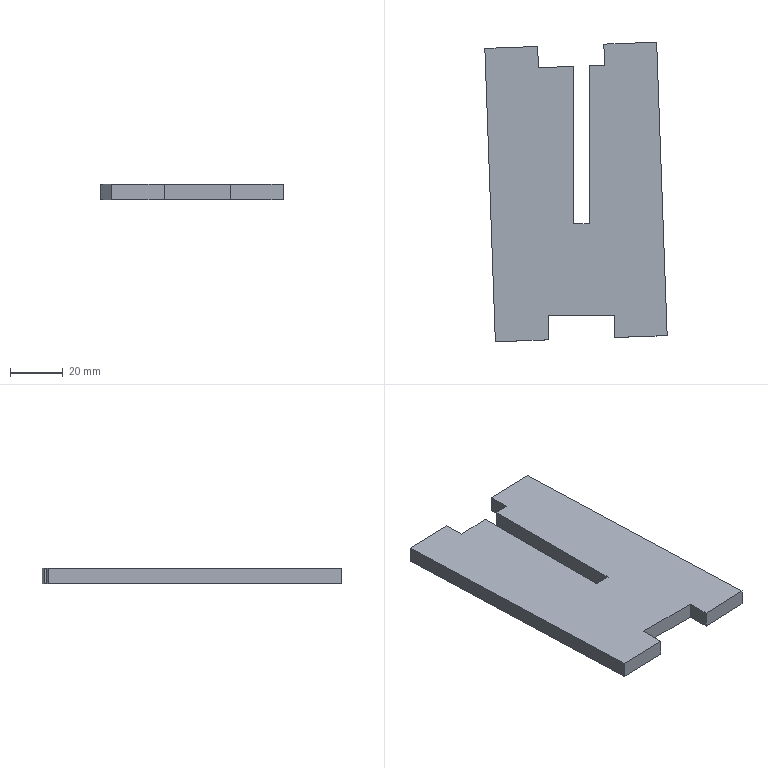Part | SolidWorks | features Extrusion 1, ICE 1 | 1 solid | 18 faces | box 68.823 x 113.082 x 6 mm | volume 38487 mm3 | plane 18
STEP:
#1=CARTESIAN_POINT('',(147.794,83.809,0.));
#2=VERTEX_POINT('',#1);
#3=CARTESIAN_POINT('',(142.029,83.603,0.));
#4=VERTEX_POINT('',#3);
#5=CARTESIAN_POINT('',(147.794,83.809,0.));
#6=DIRECTION('',(-0.9994,-0.03577,0.));
#7=VECTOR('',#6,1000.);
#8=LINE('',#5,#7);
#9=EDGE_CURVE('',#2,#4,#8,.T.);
#10=ORIENTED_EDGE('',*,*,#9,.T.);
#11=CARTESIAN_POINT('',(142.029,83.603,6.));
#12=VERTEX_POINT('',#11);
#13=CARTESIAN_POINT('',(142.029,83.603,6.));
#14=DIRECTION('',(0.,0.,1.));
#15=VECTOR('',#14,1000.);
#16=LINE('',#13,#15);
#17=EDGE_CURVE('',#4,#12,#16,.T.);
#18=ORIENTED_EDGE('',*,*,#17,.T.);
#19=CARTESIAN_POINT('',(147.794,83.809,6.));
#20=VERTEX_POINT('',#19);
#21=CARTESIAN_POINT('',(147.794,83.809,6.));
#22=DIRECTION('',(-0.9994,-0.03577,0.));
#23=VECTOR('',#22,1000.);
#24=LINE('',#21,#23);
#25=EDGE_CURVE('',#20,#12,#24,.T.);
#26=ORIENTED_EDGE('',*,*,#25,.F.);
#27=CARTESIAN_POINT('',(147.794,83.809,6.));
#28=DIRECTION('',(0.,0.,-1.));
#29=VECTOR('',#28,1000.);
#30=LINE('',#27,#29);
#31=EDGE_CURVE('',#20,#2,#30,.T.);
#32=ORIENTED_EDGE('',*,*,#31,.T.);
#33=EDGE_LOOP('',(#10,#18,#26,#32));
#34=FACE_OUTER_BOUND('',#33,.T.);
#35=CARTESIAN_POINT('',(147.794,83.809,6.));
#36=DIRECTION('',(0.03577,-0.9994,0.));
#37=DIRECTION('',(0.9994,0.03577,0.));
#38=AXIS2_PLACEMENT_3D('',#35,#36,#37);
#39=PLANE('',#38);
#40=ADVANCED_FACE('',(#34),#39,.F.);
#41=CARTESIAN_POINT('',(136.029,83.388,6.));
#42=VERTEX_POINT('',#41);
#43=CARTESIAN_POINT('',(122.81,82.915,6.));
#44=VERTEX_POINT('',#43);
#45=CARTESIAN_POINT('',(147.794,83.809,6.));
#46=DIRECTION('',(-0.9994,-0.03577,0.));
#47=VECTOR('',#46,1000.);
#48=LINE('',#45,#47);
#49=EDGE_CURVE('',#42,#44,#48,.T.);
#50=ORIENTED_EDGE('',*,*,#49,.F.);
#51=CARTESIAN_POINT('',(136.029,83.388,0.));
#52=VERTEX_POINT('',#51);
#53=CARTESIAN_POINT('',(136.029,83.388,6.));
#54=DIRECTION('',(0.,0.,-1.));
#55=VECTOR('',#54,1000.);
#56=LINE('',#53,#55);
#57=EDGE_CURVE('',#42,#52,#56,.T.);
#58=ORIENTED_EDGE('',*,*,#57,.T.);
#59=CARTESIAN_POINT('',(122.81,82.915,0.));
#60=VERTEX_POINT('',#59);
#61=CARTESIAN_POINT('',(147.794,83.809,0.));
#62=DIRECTION('',(-0.9994,-0.03577,0.));
#63=VECTOR('',#62,1000.);
#64=LINE('',#61,#63);
#65=EDGE_CURVE('',#52,#60,#64,.T.);
#66=ORIENTED_EDGE('',*,*,#65,.T.);
#67=CARTESIAN_POINT('',(122.81,82.915,6.));
#68=DIRECTION('',(0.,0.,-1.));
#69=VECTOR('',#68,1000.);
#70=LINE('',#67,#69);
#71=EDGE_CURVE('',#44,#60,#70,.T.);
#72=ORIENTED_EDGE('',*,*,#71,.F.);
#73=EDGE_LOOP('',(#50,#58,#66,#72));
#74=FACE_OUTER_BOUND('',#73,.T.);
#75=CARTESIAN_POINT('',(147.794,83.809,6.));
#76=DIRECTION('',(0.03577,-0.9994,0.));
#77=DIRECTION('',(0.9994,0.03577,0.));
#78=AXIS2_PLACEMENT_3D('',#75,#76,#77);
#79=PLANE('',#78);
#80=ADVANCED_FACE('',(#74),#79,.F.);
#81=CARTESIAN_POINT('',(122.524,90.91,0.));
#82=VERTEX_POINT('',#81);
#83=CARTESIAN_POINT('',(122.81,82.915,0.));
#84=DIRECTION('',(-0.03577,0.9994,0.));
#85=VECTOR('',#84,1000.);
#86=LINE('',#83,#85);
#87=EDGE_CURVE('',#60,#82,#86,.T.);
#88=ORIENTED_EDGE('',*,*,#87,.T.);
#89=CARTESIAN_POINT('',(122.524,90.91,6.));
#90=VERTEX_POINT('',#89);
#91=CARTESIAN_POINT('',(122.524,90.91,6.));
#92=DIRECTION('',(0.,0.,-1.));
#93=VECTOR('',#92,1000.);
#94=LINE('',#91,#93);
#95=EDGE_CURVE('',#90,#82,#94,.T.);
#96=ORIENTED_EDGE('',*,*,#95,.F.);
#97=CARTESIAN_POINT('',(122.81,82.915,6.));
#98=DIRECTION('',(-0.03577,0.9994,0.));
#99=VECTOR('',#98,1000.);
#100=LINE('',#97,#99);
#101=EDGE_CURVE('',#44,#90,#100,.T.);
#102=ORIENTED_EDGE('',*,*,#101,.F.);
#103=ORIENTED_EDGE('',*,*,#71,.T.);
#104=EDGE_LOOP('',(#88,#96,#102,#103));
#105=FACE_OUTER_BOUND('',#104,.T.);
#106=CARTESIAN_POINT('',(122.81,82.915,6.));
#107=DIRECTION('',(-0.9994,-0.03577,0.));
#108=DIRECTION('',(0.03577,-0.9994,0.));
#109=AXIS2_PLACEMENT_3D('',#106,#107,#108);
#110=PLANE('',#109);
#111=ADVANCED_FACE('',(#105),#110,.F.);
#112=CARTESIAN_POINT('',(102.587,90.196,0.));
#113=VERTEX_POINT('',#112);
#114=CARTESIAN_POINT('',(122.524,90.91,0.));
#115=DIRECTION('',(-0.9994,-0.03577,0.));
#116=VECTOR('',#115,1000.);
#117=LINE('',#114,#116);
#118=EDGE_CURVE('',#82,#113,#117,.T.);
#119=ORIENTED_EDGE('',*,*,#118,.T.);
#120=CARTESIAN_POINT('',(102.587,90.196,6.));
#121=VERTEX_POINT('',#120);
#122=CARTESIAN_POINT('',(102.587,90.196,6.));
#123=DIRECTION('',(0.,0.,-1.));
#124=VECTOR('',#123,1000.);
#125=LINE('',#122,#124);
#126=EDGE_CURVE('',#121,#113,#125,.T.);
#127=ORIENTED_EDGE('',*,*,#126,.F.);
#128=CARTESIAN_POINT('',(122.524,90.91,6.));
#129=DIRECTION('',(-0.9994,-0.03577,0.));
#130=VECTOR('',#129,1000.);
#131=LINE('',#128,#130);
#132=EDGE_CURVE('',#90,#121,#131,.T.);
#133=ORIENTED_EDGE('',*,*,#132,.F.);
#134=ORIENTED_EDGE('',*,*,#95,.T.);
#135=EDGE_LOOP('',(#119,#127,#133,#134));
#136=FACE_OUTER_BOUND('',#135,.T.);
#137=CARTESIAN_POINT('',(122.524,90.91,6.));
#138=DIRECTION('',(0.03577,-0.9994,0.));
#139=DIRECTION('',(0.9994,0.03577,0.));
#140=AXIS2_PLACEMENT_3D('',#137,#138,#139);
#141=PLANE('',#140);
#142=ADVANCED_FACE('',(#136),#141,.F.);
#143=CARTESIAN_POINT('',(106.552,-20.564,0.));
#144=VERTEX_POINT('',#143);
#145=CARTESIAN_POINT('',(106.552,-20.564,0.));
#146=DIRECTION('',(0.03577,-0.9994,0.));
#147=VECTOR('',#146,1000.);
#148=LINE('',#145,#147);
#149=EDGE_CURVE('',#113,#144,#148,.T.);
#150=ORIENTED_EDGE('',*,*,#149,.T.);
#151=CARTESIAN_POINT('',(106.552,-20.564,6.));
#152=VERTEX_POINT('',#151);
#153=CARTESIAN_POINT('',(106.552,-20.564,6.));
#154=DIRECTION('',(0.,0.,-1.));
#155=VECTOR('',#154,1000.);
#156=LINE('',#153,#155);
#157=EDGE_CURVE('',#152,#144,#156,.T.);
#158=ORIENTED_EDGE('',*,*,#157,.F.);
#159=CARTESIAN_POINT('',(106.552,-20.564,6.));
#160=DIRECTION('',(0.03577,-0.9994,0.));
#161=VECTOR('',#160,1000.);
#162=LINE('',#159,#161);
#163=EDGE_CURVE('',#121,#152,#162,.T.);
#164=ORIENTED_EDGE('',*,*,#163,.F.);
#165=ORIENTED_EDGE('',*,*,#126,.T.);
#166=EDGE_LOOP('',(#150,#158,#164,#165));
#167=FACE_OUTER_BOUND('',#166,.T.);
#168=CARTESIAN_POINT('',(106.552,-20.564,6.));
#169=DIRECTION('',(0.9994,0.03577,0.));
#170=DIRECTION('',(-0.03577,0.9994,0.));
#171=AXIS2_PLACEMENT_3D('',#168,#169,#170);
#172=PLANE('',#171);
#173=ADVANCED_FACE('',(#167),#172,.F.);
#174=CARTESIAN_POINT('',(126.528,-19.849,0.));
#175=VERTEX_POINT('',#174);
#176=CARTESIAN_POINT('',(106.552,-20.564,0.));
#177=DIRECTION('',(0.9994,0.03577,0.));
#178=VECTOR('',#177,1000.);
#179=LINE('',#176,#178);
#180=EDGE_CURVE('',#144,#175,#179,.T.);
#181=ORIENTED_EDGE('',*,*,#180,.T.);
#182=CARTESIAN_POINT('',(126.528,-19.849,6.));
#183=VERTEX_POINT('',#182);
#184=CARTESIAN_POINT('',(126.528,-19.849,6.));
#185=DIRECTION('',(0.,0.,-1.));
#186=VECTOR('',#185,1000.);
#187=LINE('',#184,#186);
#188=EDGE_CURVE('',#183,#175,#187,.T.);
#189=ORIENTED_EDGE('',*,*,#188,.F.);
#190=CARTESIAN_POINT('',(106.552,-20.564,6.));
#191=DIRECTION('',(0.9994,0.03577,0.));
#192=VECTOR('',#191,1000.);
#193=LINE('',#190,#192);
#194=EDGE_CURVE('',#152,#183,#193,.T.);
#195=ORIENTED_EDGE('',*,*,#194,.F.);
#196=ORIENTED_EDGE('',*,*,#157,.T.);
#197=EDGE_LOOP('',(#181,#189,#195,#196));
#198=FACE_OUTER_BOUND('',#197,.T.);
#199=CARTESIAN_POINT('',(106.552,-20.564,6.));
#200=DIRECTION('',(-0.03577,0.9994,0.));
#201=DIRECTION('',(-0.9994,-0.03577,0.));
#202=AXIS2_PLACEMENT_3D('',#199,#200,#201);
#203=PLANE('',#202);
#204=ADVANCED_FACE('',(#198),#203,.F.);
#205=CARTESIAN_POINT('',(126.528,-10.564,0.));
#206=VERTEX_POINT('',#205);
#207=CARTESIAN_POINT('',(126.528,-19.849,0.));
#208=DIRECTION('',(0.,1.,0.));
#209=VECTOR('',#208,1000.);
#210=LINE('',#207,#209);
#211=EDGE_CURVE('',#175,#206,#210,.T.);
#212=ORIENTED_EDGE('',*,*,#211,.T.);
#213=CARTESIAN_POINT('',(126.528,-10.564,6.));
#214=VERTEX_POINT('',#213);
#215=CARTESIAN_POINT('',(126.528,-10.564,6.));
#216=DIRECTION('',(0.,0.,-1.));
#217=VECTOR('',#216,1000.);
#218=LINE('',#215,#217);
#219=EDGE_CURVE('',#214,#206,#218,.T.);
#220=ORIENTED_EDGE('',*,*,#219,.F.);
#221=CARTESIAN_POINT('',(126.528,-19.849,6.));
#222=DIRECTION('',(0.,1.,0.));
#223=VECTOR('',#222,1000.);
#224=LINE('',#221,#223);
#225=EDGE_CURVE('',#183,#214,#224,.T.);
#226=ORIENTED_EDGE('',*,*,#225,.F.);
#227=ORIENTED_EDGE('',*,*,#188,.T.);
#228=EDGE_LOOP('',(#212,#220,#226,#227));
#229=FACE_OUTER_BOUND('',#228,.T.);
#230=CARTESIAN_POINT('',(126.528,-19.849,6.));
#231=DIRECTION('',(-1.,0.,0.));
#232=DIRECTION('',(0.,0.,1.));
#233=AXIS2_PLACEMENT_3D('',#230,#231,#232);
#234=PLANE('',#233);
#235=ADVANCED_FACE('',(#229),#234,.F.);
#236=CARTESIAN_POINT('',(151.529,-10.564,0.));
#237=VERTEX_POINT('',#236);
#238=CARTESIAN_POINT('',(126.528,-10.564,0.));
#239=DIRECTION('',(1.,0.,0.));
#240=VECTOR('',#239,1000.);
#241=LINE('',#238,#240);
#242=EDGE_CURVE('',#206,#237,#241,.T.);
#243=ORIENTED_EDGE('',*,*,#242,.T.);
#244=CARTESIAN_POINT('',(151.529,-10.564,6.));
#245=VERTEX_POINT('',#244);
#246=CARTESIAN_POINT('',(151.529,-10.564,6.));
#247=DIRECTION('',(0.,0.,-1.));
#248=VECTOR('',#247,1000.);
#249=LINE('',#246,#248);
#250=EDGE_CURVE('',#245,#237,#249,.T.);
#251=ORIENTED_EDGE('',*,*,#250,.F.);
#252=CARTESIAN_POINT('',(126.528,-10.564,6.));
#253=DIRECTION('',(1.,0.,0.));
#254=VECTOR('',#253,1000.);
#255=LINE('',#252,#254);
#256=EDGE_CURVE('',#214,#245,#255,.T.);
#257=ORIENTED_EDGE('',*,*,#256,.F.);
#258=ORIENTED_EDGE('',*,*,#219,.T.);
#259=EDGE_LOOP('',(#243,#251,#257,#258));
#260=FACE_OUTER_BOUND('',#259,.T.);
#261=CARTESIAN_POINT('',(126.528,-10.564,6.));
#262=DIRECTION('',(0.,1.,0.));
#263=DIRECTION('',(-1.,0.,0.));
#264=AXIS2_PLACEMENT_3D('',#261,#262,#263);
#265=PLANE('',#264);
#266=ADVANCED_FACE('',(#260),#265,.F.);
#267=CARTESIAN_POINT('',(151.529,-18.954,0.));
#268=VERTEX_POINT('',#267);
#269=CARTESIAN_POINT('',(151.529,-10.564,0.));
#270=DIRECTION('',(0.,-1.,0.));
#271=VECTOR('',#270,1000.);
#272=LINE('',#269,#271);
#273=EDGE_CURVE('',#237,#268,#272,.T.);
#274=ORIENTED_EDGE('',*,*,#273,.T.);
#275=CARTESIAN_POINT('',(151.529,-18.954,6.));
#276=VERTEX_POINT('',#275);
#277=CARTESIAN_POINT('',(151.529,-18.954,6.));
#278=DIRECTION('',(0.,0.,-1.));
#279=VECTOR('',#278,1000.);
#280=LINE('',#277,#279);
#281=EDGE_CURVE('',#276,#268,#280,.T.);
#282=ORIENTED_EDGE('',*,*,#281,.F.);
#283=CARTESIAN_POINT('',(151.529,-10.564,6.));
#284=DIRECTION('',(0.,-1.,0.));
#285=VECTOR('',#284,1000.);
#286=LINE('',#283,#285);
#287=EDGE_CURVE('',#245,#276,#286,.T.);
#288=ORIENTED_EDGE('',*,*,#287,.F.);
#289=ORIENTED_EDGE('',*,*,#250,.T.);
#290=EDGE_LOOP('',(#274,#282,#288,#289));
#291=FACE_OUTER_BOUND('',#290,.T.);
#292=CARTESIAN_POINT('',(151.529,-10.564,6.));
#293=DIRECTION('',(1.,0.,0.));
#294=DIRECTION('',(0.,0.,-1.));
#295=AXIS2_PLACEMENT_3D('',#292,#293,#294);
#296=PLANE('',#295);
#297=ADVANCED_FACE('',(#291),#296,.F.);
#298=CARTESIAN_POINT('',(171.41,-18.242,0.));
#299=VERTEX_POINT('',#298);
#300=CARTESIAN_POINT('',(151.529,-18.954,0.));
#301=DIRECTION('',(0.9994,0.03577,0.));
#302=VECTOR('',#301,1000.);
#303=LINE('',#300,#302);
#304=EDGE_CURVE('',#268,#299,#303,.T.);
#305=ORIENTED_EDGE('',*,*,#304,.T.);
#306=CARTESIAN_POINT('',(171.41,-18.242,6.));
#307=VERTEX_POINT('',#306);
#308=CARTESIAN_POINT('',(171.41,-18.242,6.));
#309=DIRECTION('',(0.,0.,-1.));
#310=VECTOR('',#309,1000.);
#311=LINE('',#308,#310);
#312=EDGE_CURVE('',#307,#299,#311,.T.);
#313=ORIENTED_EDGE('',*,*,#312,.F.);
#314=CARTESIAN_POINT('',(151.529,-18.954,6.));
#315=DIRECTION('',(0.9994,0.03577,0.));
#316=VECTOR('',#315,1000.);
#317=LINE('',#314,#316);
#318=EDGE_CURVE('',#276,#307,#317,.T.);
#319=ORIENTED_EDGE('',*,*,#318,.F.);
#320=ORIENTED_EDGE('',*,*,#281,.T.);
#321=EDGE_LOOP('',(#305,#313,#319,#320));
#322=FACE_OUTER_BOUND('',#321,.T.);
#323=CARTESIAN_POINT('',(151.529,-18.954,6.));
#324=DIRECTION('',(-0.03577,0.9994,0.));
#325=DIRECTION('',(-0.9994,-0.03577,0.));
#326=AXIS2_PLACEMENT_3D('',#323,#324,#325);
#327=PLANE('',#326);
#328=ADVANCED_FACE('',(#322),#327,.F.);
#329=CARTESIAN_POINT('',(167.445,92.518,0.));
#330=VERTEX_POINT('',#329);
#331=CARTESIAN_POINT('',(171.41,-18.242,0.));
#332=DIRECTION('',(-0.03577,0.9994,0.));
#333=VECTOR('',#332,1000.);
#334=LINE('',#331,#333);
#335=EDGE_CURVE('',#299,#330,#334,.T.);
#336=ORIENTED_EDGE('',*,*,#335,.T.);
#337=CARTESIAN_POINT('',(167.445,92.518,6.));
#338=VERTEX_POINT('',#337);
#339=CARTESIAN_POINT('',(167.445,92.518,6.));
#340=DIRECTION('',(0.,0.,-1.));
#341=VECTOR('',#340,1000.);
#342=LINE('',#339,#341);
#343=EDGE_CURVE('',#338,#330,#342,.T.);
#344=ORIENTED_EDGE('',*,*,#343,.F.);
#345=CARTESIAN_POINT('',(171.41,-18.242,6.));
#346=DIRECTION('',(-0.03577,0.9994,0.));
#347=VECTOR('',#346,1000.);
#348=LINE('',#345,#347);
#349=EDGE_CURVE('',#307,#338,#348,.T.);
#350=ORIENTED_EDGE('',*,*,#349,.F.);
#351=ORIENTED_EDGE('',*,*,#312,.T.);
#352=EDGE_LOOP('',(#336,#344,#350,#351));
#353=FACE_OUTER_BOUND('',#352,.T.);
#354=CARTESIAN_POINT('',(171.41,-18.242,6.));
#355=DIRECTION('',(-0.9994,-0.03577,0.));
#356=DIRECTION('',(0.03577,-0.9994,0.));
#357=AXIS2_PLACEMENT_3D('',#354,#355,#356);
#358=PLANE('',#357);
#359=ADVANCED_FACE('',(#353),#358,.F.);
#360=CARTESIAN_POINT('',(147.508,91.804,0.));
#361=VERTEX_POINT('',#360);
#362=CARTESIAN_POINT('',(147.508,91.804,0.));
#363=DIRECTION('',(-0.9994,-0.03577,0.));
#364=VECTOR('',#363,1000.);
#365=LINE('',#362,#364);
#366=EDGE_CURVE('',#330,#361,#365,.T.);
#367=ORIENTED_EDGE('',*,*,#366,.T.);
#368=CARTESIAN_POINT('',(147.508,91.804,6.));
#369=VERTEX_POINT('',#368);
#370=CARTESIAN_POINT('',(147.508,91.804,6.));
#371=DIRECTION('',(0.,0.,-1.));
#372=VECTOR('',#371,1000.);
#373=LINE('',#370,#372);
#374=EDGE_CURVE('',#369,#361,#373,.T.);
#375=ORIENTED_EDGE('',*,*,#374,.F.);
#376=CARTESIAN_POINT('',(147.508,91.804,6.));
#377=DIRECTION('',(-0.9994,-0.03577,0.));
#378=VECTOR('',#377,1000.);
#379=LINE('',#376,#378);
#380=EDGE_CURVE('',#338,#369,#379,.T.);
#381=ORIENTED_EDGE('',*,*,#380,.F.);
#382=ORIENTED_EDGE('',*,*,#343,.T.);
#383=EDGE_LOOP('',(#367,#375,#381,#382));
#384=FACE_OUTER_BOUND('',#383,.T.);
#385=CARTESIAN_POINT('',(147.508,91.804,6.));
#386=DIRECTION('',(0.03577,-0.9994,0.));
#387=DIRECTION('',(0.9994,0.03577,0.));
#388=AXIS2_PLACEMENT_3D('',#385,#386,#387);
#389=PLANE('',#388);
#390=ADVANCED_FACE('',(#384),#389,.F.);
#391=CARTESIAN_POINT('',(147.794,83.809,0.));
#392=DIRECTION('',(0.03577,-0.9994,0.));
#393=VECTOR('',#392,1000.);
#394=LINE('',#391,#393);
#395=EDGE_CURVE('',#361,#2,#394,.T.);
#396=ORIENTED_EDGE('',*,*,#395,.T.);
#397=ORIENTED_EDGE('',*,*,#31,.F.);
#398=CARTESIAN_POINT('',(147.794,83.809,6.));
#399=DIRECTION('',(0.03577,-0.9994,0.));
#400=VECTOR('',#399,1000.);
#401=LINE('',#398,#400);
#402=EDGE_CURVE('',#369,#20,#401,.T.);
#403=ORIENTED_EDGE('',*,*,#402,.F.);
#404=ORIENTED_EDGE('',*,*,#374,.T.);
#405=EDGE_LOOP('',(#396,#397,#403,#404));
#406=FACE_OUTER_BOUND('',#405,.T.);
#407=CARTESIAN_POINT('',(147.794,83.809,6.));
#408=DIRECTION('',(0.9994,0.03577,0.));
#409=DIRECTION('',(-0.03577,0.9994,0.));
#410=AXIS2_PLACEMENT_3D('',#407,#408,#409);
#411=PLANE('',#410);
#412=ADVANCED_FACE('',(#406),#411,.F.);
#413=ORIENTED_EDGE('',*,*,#25,.T.);
#414=CARTESIAN_POINT('',(142.029,23.91,6.));
#415=VERTEX_POINT('',#414);
#416=CARTESIAN_POINT('',(142.029,83.886,6.));
#417=DIRECTION('',(0.,1.,0.));
#418=VECTOR('',#417,1000.);
#419=LINE('',#416,#418);
#420=EDGE_CURVE('',#415,#12,#419,.T.);
#421=ORIENTED_EDGE('',*,*,#420,.F.);
#422=CARTESIAN_POINT('',(136.029,23.91,6.));
#423=VERTEX_POINT('',#422);
#424=CARTESIAN_POINT('',(136.029,23.91,6.));
#425=DIRECTION('',(1.,0.,0.));
#426=VECTOR('',#425,1000.);
#427=LINE('',#424,#426);
#428=EDGE_CURVE('',#423,#415,#427,.T.);
#429=ORIENTED_EDGE('',*,*,#428,.F.);
#430=CARTESIAN_POINT('',(136.029,83.886,6.));
#431=DIRECTION('',(0.,-1.,0.));
#432=VECTOR('',#431,1000.);
#433=LINE('',#430,#432);
#434=EDGE_CURVE('',#42,#423,#433,.T.);
#435=ORIENTED_EDGE('',*,*,#434,.F.);
#436=ORIENTED_EDGE('',*,*,#49,.T.);
#437=ORIENTED_EDGE('',*,*,#101,.T.);
#438=ORIENTED_EDGE('',*,*,#132,.T.);
#439=ORIENTED_EDGE('',*,*,#163,.T.);
#440=ORIENTED_EDGE('',*,*,#194,.T.);
#441=ORIENTED_EDGE('',*,*,#225,.T.);
#442=ORIENTED_EDGE('',*,*,#256,.T.);
#443=ORIENTED_EDGE('',*,*,#287,.T.);
#444=ORIENTED_EDGE('',*,*,#318,.T.);
#445=ORIENTED_EDGE('',*,*,#349,.T.);
#446=ORIENTED_EDGE('',*,*,#380,.T.);
#447=ORIENTED_EDGE('',*,*,#402,.T.);
#448=EDGE_LOOP('',(#413,#421,#429,#435,#436,#437,#438,#439,#440,#441,#442,#443,#444,#445,#446,#447));
#449=FACE_OUTER_BOUND('',#448,.T.);
#450=CARTESIAN_POINT('',(0.,0.,6.));
#451=DIRECTION('',(0.,0.,-1.));
#452=DIRECTION('',(-1.,0.,0.));
#453=AXIS2_PLACEMENT_3D('',#450,#451,#452);
#454=PLANE('',#453);
#455=ADVANCED_FACE('',(#449),#454,.F.);
#456=CARTESIAN_POINT('',(142.029,23.91,0.));
#457=VERTEX_POINT('',#456);
#458=CARTESIAN_POINT('',(142.029,83.886,0.));
#459=DIRECTION('',(0.,1.,0.));
#460=VECTOR('',#459,1000.);
#461=LINE('',#458,#460);
#462=EDGE_CURVE('',#457,#4,#461,.T.);
#463=ORIENTED_EDGE('',*,*,#462,.T.);
#464=ORIENTED_EDGE('',*,*,#9,.F.);
#465=ORIENTED_EDGE('',*,*,#395,.F.);
#466=ORIENTED_EDGE('',*,*,#366,.F.);
#467=ORIENTED_EDGE('',*,*,#335,.F.);
#468=ORIENTED_EDGE('',*,*,#304,.F.);
#469=ORIENTED_EDGE('',*,*,#273,.F.);
#470=ORIENTED_EDGE('',*,*,#242,.F.);
#471=ORIENTED_EDGE('',*,*,#211,.F.);
#472=ORIENTED_EDGE('',*,*,#180,.F.);
#473=ORIENTED_EDGE('',*,*,#149,.F.);
#474=ORIENTED_EDGE('',*,*,#118,.F.);
#475=ORIENTED_EDGE('',*,*,#87,.F.);
#476=ORIENTED_EDGE('',*,*,#65,.F.);
#477=CARTESIAN_POINT('',(136.029,23.91,0.));
#478=VERTEX_POINT('',#477);
#479=CARTESIAN_POINT('',(136.029,0.,0.));
#480=DIRECTION('',(0.,1.,0.));
#481=VECTOR('',#480,1000.);
#482=LINE('',#479,#481);
#483=EDGE_CURVE('',#478,#52,#482,.T.);
#484=ORIENTED_EDGE('',*,*,#483,.F.);
#485=CARTESIAN_POINT('',(136.029,23.91,0.));
#486=DIRECTION('',(1.,0.,0.));
#487=VECTOR('',#486,1000.);
#488=LINE('',#485,#487);
#489=EDGE_CURVE('',#478,#457,#488,.T.);
#490=ORIENTED_EDGE('',*,*,#489,.T.);
#491=EDGE_LOOP('',(#463,#464,#465,#466,#467,#468,#469,#470,#471,#472,#473,#474,#475,#476,#484,#490));
#492=FACE_OUTER_BOUND('',#491,.T.);
#493=CARTESIAN_POINT('',(0.,0.,0.));
#494=DIRECTION('',(0.,0.,-1.));
#495=DIRECTION('',(-1.,0.,0.));
#496=AXIS2_PLACEMENT_3D('',#493,#494,#495);
#497=PLANE('',#496);
#498=ADVANCED_FACE('',(#492),#497,.T.);
#499=ORIENTED_EDGE('',*,*,#462,.F.);
#500=CARTESIAN_POINT('',(142.029,23.91,0.));
#501=DIRECTION('',(0.,0.,1.));
#502=VECTOR('',#501,1000.);
#503=LINE('',#500,#502);
#504=EDGE_CURVE('',#457,#415,#503,.T.);
#505=ORIENTED_EDGE('',*,*,#504,.T.);
#506=ORIENTED_EDGE('',*,*,#420,.T.);
#507=ORIENTED_EDGE('',*,*,#17,.F.);
#508=EDGE_LOOP('',(#499,#505,#506,#507));
#509=FACE_OUTER_BOUND('',#508,.T.);
#510=CARTESIAN_POINT('',(142.029,83.886,0.));
#511=DIRECTION('',(1.,0.,0.));
#512=DIRECTION('',(0.,0.,-1.));
#513=AXIS2_PLACEMENT_3D('',#510,#511,#512);
#514=PLANE('',#513);
#515=ADVANCED_FACE('',(#509),#514,.F.);
#516=ORIENTED_EDGE('',*,*,#434,.T.);
#517=CARTESIAN_POINT('',(136.029,23.91,0.));
#518=DIRECTION('',(0.,0.,1.));
#519=VECTOR('',#518,1000.);
#520=LINE('',#517,#519);
#521=EDGE_CURVE('',#478,#423,#520,.T.);
#522=ORIENTED_EDGE('',*,*,#521,.F.);
#523=ORIENTED_EDGE('',*,*,#483,.T.);
#524=ORIENTED_EDGE('',*,*,#57,.F.);
#525=EDGE_LOOP('',(#516,#522,#523,#524));
#526=FACE_OUTER_BOUND('',#525,.T.);
#527=CARTESIAN_POINT('',(136.029,83.886,0.));
#528=DIRECTION('',(-1.,0.,0.));
#529=DIRECTION('',(0.,0.,1.));
#530=AXIS2_PLACEMENT_3D('',#527,#528,#529);
#531=PLANE('',#530);
#532=ADVANCED_FACE('',(#526),#531,.F.);
#533=ORIENTED_EDGE('',*,*,#428,.T.);
#534=ORIENTED_EDGE('',*,*,#504,.F.);
#535=ORIENTED_EDGE('',*,*,#489,.F.);
#536=ORIENTED_EDGE('',*,*,#521,.T.);
#537=EDGE_LOOP('',(#533,#534,#535,#536));
#538=FACE_OUTER_BOUND('',#537,.T.);
#539=CARTESIAN_POINT('',(136.029,23.91,0.));
#540=DIRECTION('',(0.,-1.,0.));
#541=DIRECTION('',(0.,0.,-1.));
#542=AXIS2_PLACEMENT_3D('',#539,#540,#541);
#543=PLANE('',#542);
#544=ADVANCED_FACE('',(#538),#543,.F.);
#545=CLOSED_SHELL('',(#40,#80,#111,#142,#173,#204,#235,#266,#297,#328,#359,#390,#412,#455,#498,#515,#532,#544));
#546=MANIFOLD_SOLID_BREP('',#545);
#547=CARTESIAN_POINT('',(0.,0.,0.));
#548=DIRECTION('',(0.,0.,1.));
#549=DIRECTION('',(1.,0.,0.));
#550=AXIS2_PLACEMENT_3D('',#547,#548,#549);
#551=(LENGTH_UNIT()NAMED_UNIT(*)SI_UNIT(.MILLI.,.METRE.));
#552=UNCERTAINTY_MEASURE_WITH_UNIT(LENGTH_MEASURE(0.00001),#551,'','');
#553=(NAMED_UNIT(*)PLANE_ANGLE_UNIT()SI_UNIT($,.RADIAN.));
#554=(NAMED_UNIT(*)SI_UNIT($,.STERADIAN.)SOLID_ANGLE_UNIT());
#555=(GEOMETRIC_REPRESENTATION_CONTEXT(3)GLOBAL_UNCERTAINTY_ASSIGNED_CONTEXT((#552))GLOBAL_UNIT_ASSIGNED_CONTEXT((#551,#553,#554))REPRESENTATION_CONTEXT('',''));
#556=ADVANCED_BREP_SHAPE_REPRESENTATION('',(#546,#550),#555);